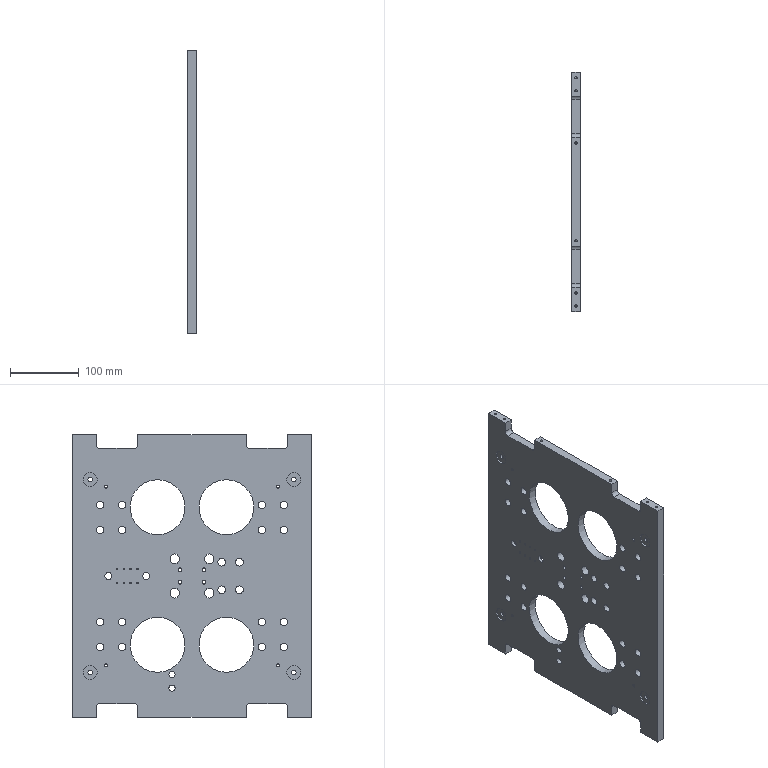Part | NX | 1 solid | 147 faces | box 12 x 348 x 411 mm | volume 1356557 mm3 | cylinder 92 | plane 43 | cone 12 | commonest cylinder face diameters 11 x24 10 x18 3.3 x12 2.5 x8 4.2 x4 5.5 x4